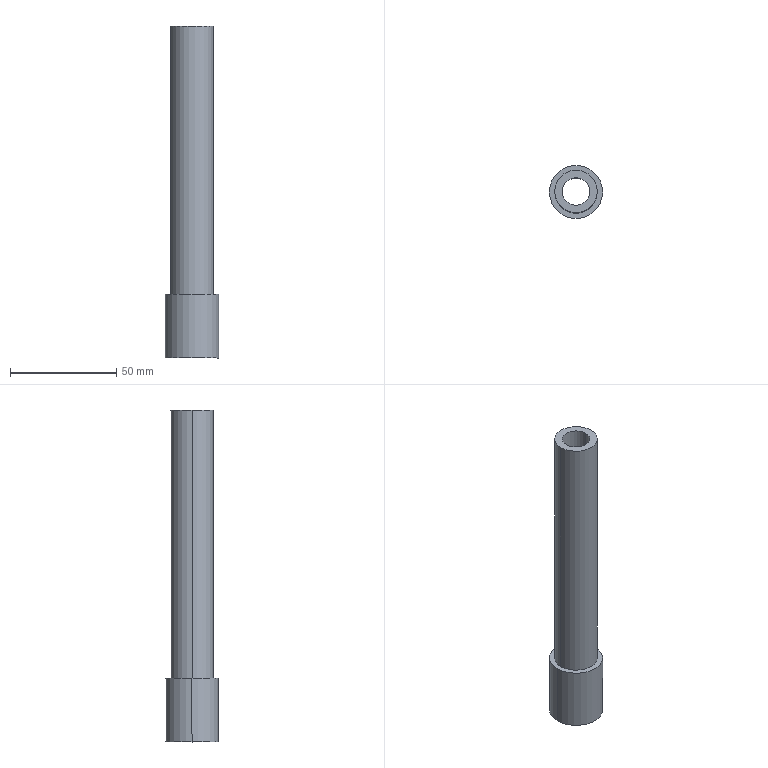Part | SolidWorks | features BaseBody 1 | 1 solid | 9 faces | box 25 x 25 x 156 mm | volume 33604 mm3 | cylinder 6 | plane 3 | commonest cylinder face diameters 13 x2 20 x2 25 x2
STEP:
#1=CARTESIAN_POINT('',(6.5,0.,78.));
#2=VERTEX_POINT('',#1);
#3=CARTESIAN_POINT('',(6.5,0.,-78.));
#4=VERTEX_POINT('',#3);
#5=CARTESIAN_POINT('',(6.5,0.,78.));
#6=DIRECTION('',(0.,0.,-1.));
#7=VECTOR('',#6,1000.);
#8=LINE('',#5,#7);
#9=EDGE_CURVE('',#2,#4,#8,.T.);
#10=ORIENTED_EDGE('',*,*,#9,.F.);
#11=CARTESIAN_POINT('',(-6.5,0.,78.));
#12=VERTEX_POINT('',#11);
#13=CARTESIAN_POINT('',(0.,0.,78.));
#14=DIRECTION('',(0.,0.,-1.));
#15=DIRECTION('',(-1.,0.,0.));
#16=AXIS2_PLACEMENT_3D('',#13,#14,#15);
#17=CIRCLE('',#16,6.5);
#18=EDGE_CURVE('',#12,#2,#17,.T.);
#19=ORIENTED_EDGE('',*,*,#18,.F.);
#20=CARTESIAN_POINT('',(-6.5,0.,-78.));
#21=VERTEX_POINT('',#20);
#22=CARTESIAN_POINT('',(-6.5,0.,78.));
#23=DIRECTION('',(0.,0.,-1.));
#24=VECTOR('',#23,1000.);
#25=LINE('',#22,#24);
#26=EDGE_CURVE('',#12,#21,#25,.T.);
#27=ORIENTED_EDGE('',*,*,#26,.T.);
#28=CARTESIAN_POINT('',(0.,0.,-78.));
#29=DIRECTION('',(0.,0.,-1.));
#30=DIRECTION('',(-1.,0.,0.));
#31=AXIS2_PLACEMENT_3D('',#28,#29,#30);
#32=CIRCLE('',#31,6.5);
#33=EDGE_CURVE('',#21,#4,#32,.T.);
#34=ORIENTED_EDGE('',*,*,#33,.T.);
#35=EDGE_LOOP('',(#10,#19,#27,#34));
#36=FACE_OUTER_BOUND('',#35,.T.);
#37=CARTESIAN_POINT('',(0.,0.,78.));
#38=DIRECTION('',(0.,0.,-1.));
#39=DIRECTION('',(-1.,0.,0.));
#40=AXIS2_PLACEMENT_3D('',#37,#38,#39);
#41=CYLINDRICAL_SURFACE('',#40,6.5);
#42=ADVANCED_FACE('',(#36),#41,.F.);
#43=ORIENTED_EDGE('',*,*,#33,.F.);
#44=CARTESIAN_POINT('',(0.,0.,-78.));
#45=DIRECTION('',(0.,0.,-1.));
#46=DIRECTION('',(-1.,0.,0.));
#47=AXIS2_PLACEMENT_3D('',#44,#45,#46);
#48=CIRCLE('',#47,6.5);
#49=EDGE_CURVE('',#4,#21,#48,.T.);
#50=ORIENTED_EDGE('',*,*,#49,.F.);
#51=EDGE_LOOP('',(#43,#50));
#52=FACE_BOUND('',#51,.T.);
#53=CARTESIAN_POINT('',(-12.5,0.,-78.));
#54=VERTEX_POINT('',#53);
#55=CARTESIAN_POINT('',(12.5,0.,-78.));
#56=VERTEX_POINT('',#55);
#57=CARTESIAN_POINT('',(0.,0.,-78.));
#58=DIRECTION('',(0.,0.,-1.));
#59=DIRECTION('',(-1.,0.,0.));
#60=AXIS2_PLACEMENT_3D('',#57,#58,#59);
#61=CIRCLE('',#60,12.5);
#62=EDGE_CURVE('',#54,#56,#61,.T.);
#63=ORIENTED_EDGE('',*,*,#62,.T.);
#64=CARTESIAN_POINT('',(0.,0.,-78.));
#65=DIRECTION('',(0.,0.,-1.));
#66=DIRECTION('',(-1.,0.,0.));
#67=AXIS2_PLACEMENT_3D('',#64,#65,#66);
#68=CIRCLE('',#67,12.5);
#69=EDGE_CURVE('',#56,#54,#68,.T.);
#70=ORIENTED_EDGE('',*,*,#69,.T.);
#71=EDGE_LOOP('',(#63,#70));
#72=FACE_OUTER_BOUND('',#71,.T.);
#73=CARTESIAN_POINT('',(0.,0.,-78.));
#74=DIRECTION('',(0.,0.,1.));
#75=DIRECTION('',(1.,0.,0.));
#76=AXIS2_PLACEMENT_3D('',#73,#74,#75);
#77=PLANE('',#76);
#78=ADVANCED_FACE('',(#52,#72),#77,.F.);
#79=CARTESIAN_POINT('',(-10.,0.,-48.));
#80=VERTEX_POINT('',#79);
#81=CARTESIAN_POINT('',(10.,0.,-48.));
#82=VERTEX_POINT('',#81);
#83=CARTESIAN_POINT('',(0.,0.,-48.));
#84=DIRECTION('',(0.,0.,-1.));
#85=DIRECTION('',(-1.,0.,0.));
#86=AXIS2_PLACEMENT_3D('',#83,#84,#85);
#87=CIRCLE('',#86,10.);
#88=EDGE_CURVE('',#80,#82,#87,.T.);
#89=ORIENTED_EDGE('',*,*,#88,.T.);
#90=CARTESIAN_POINT('',(0.,0.,-48.));
#91=DIRECTION('',(0.,0.,-1.));
#92=DIRECTION('',(-1.,0.,0.));
#93=AXIS2_PLACEMENT_3D('',#90,#91,#92);
#94=CIRCLE('',#93,10.);
#95=EDGE_CURVE('',#82,#80,#94,.T.);
#96=ORIENTED_EDGE('',*,*,#95,.T.);
#97=EDGE_LOOP('',(#89,#96));
#98=FACE_BOUND('',#97,.T.);
#99=CARTESIAN_POINT('',(-12.5,0.,-48.));
#100=VERTEX_POINT('',#99);
#101=CARTESIAN_POINT('',(12.5,0.,-48.));
#102=VERTEX_POINT('',#101);
#103=CARTESIAN_POINT('',(0.,0.,-48.));
#104=DIRECTION('',(0.,0.,-1.));
#105=DIRECTION('',(-1.,0.,0.));
#106=AXIS2_PLACEMENT_3D('',#103,#104,#105);
#107=CIRCLE('',#106,12.5);
#108=EDGE_CURVE('',#100,#102,#107,.T.);
#109=ORIENTED_EDGE('',*,*,#108,.F.);
#110=CARTESIAN_POINT('',(0.,0.,-48.));
#111=DIRECTION('',(0.,0.,-1.));
#112=DIRECTION('',(-1.,0.,0.));
#113=AXIS2_PLACEMENT_3D('',#110,#111,#112);
#114=CIRCLE('',#113,12.5);
#115=EDGE_CURVE('',#102,#100,#114,.T.);
#116=ORIENTED_EDGE('',*,*,#115,.F.);
#117=EDGE_LOOP('',(#109,#116));
#118=FACE_OUTER_BOUND('',#117,.T.);
#119=CARTESIAN_POINT('',(0.,0.,-48.));
#120=DIRECTION('',(0.,0.,-1.));
#121=DIRECTION('',(0.,-1.,0.));
#122=AXIS2_PLACEMENT_3D('',#119,#120,#121);
#123=PLANE('',#122);
#124=ADVANCED_FACE('',(#98,#118),#123,.F.);
#125=CARTESIAN_POINT('',(12.5,0.,-48.));
#126=DIRECTION('',(0.,0.,-1.));
#127=VECTOR('',#126,1000.);
#128=LINE('',#125,#127);
#129=EDGE_CURVE('',#102,#56,#128,.T.);
#130=ORIENTED_EDGE('',*,*,#129,.F.);
#131=ORIENTED_EDGE('',*,*,#115,.T.);
#132=CARTESIAN_POINT('',(-12.5,0.,-48.));
#133=DIRECTION('',(0.,0.,-1.));
#134=VECTOR('',#133,1000.);
#135=LINE('',#132,#134);
#136=EDGE_CURVE('',#100,#54,#135,.T.);
#137=ORIENTED_EDGE('',*,*,#136,.T.);
#138=ORIENTED_EDGE('',*,*,#69,.F.);
#139=EDGE_LOOP('',(#130,#131,#137,#138));
#140=FACE_OUTER_BOUND('',#139,.T.);
#141=CARTESIAN_POINT('',(0.,0.,-48.));
#142=DIRECTION('',(0.,0.,-1.));
#143=DIRECTION('',(-1.,0.,0.));
#144=AXIS2_PLACEMENT_3D('',#141,#142,#143);
#145=CYLINDRICAL_SURFACE('',#144,12.5);
#146=ADVANCED_FACE('',(#140),#145,.T.);
#147=ORIENTED_EDGE('',*,*,#18,.T.);
#148=CARTESIAN_POINT('',(0.,0.,78.));
#149=DIRECTION('',(0.,0.,-1.));
#150=DIRECTION('',(-1.,0.,0.));
#151=AXIS2_PLACEMENT_3D('',#148,#149,#150);
#152=CIRCLE('',#151,6.5);
#153=EDGE_CURVE('',#2,#12,#152,.T.);
#154=ORIENTED_EDGE('',*,*,#153,.T.);
#155=EDGE_LOOP('',(#147,#154));
#156=FACE_BOUND('',#155,.T.);
#157=CARTESIAN_POINT('',(-10.,0.,78.));
#158=VERTEX_POINT('',#157);
#159=CARTESIAN_POINT('',(10.,0.,78.));
#160=VERTEX_POINT('',#159);
#161=CARTESIAN_POINT('',(0.,0.,78.));
#162=DIRECTION('',(0.,0.,1.));
#163=DIRECTION('',(1.,0.,0.));
#164=AXIS2_PLACEMENT_3D('',#161,#162,#163);
#165=CIRCLE('',#164,10.);
#166=EDGE_CURVE('',#158,#160,#165,.T.);
#167=ORIENTED_EDGE('',*,*,#166,.T.);
#168=CARTESIAN_POINT('',(0.,0.,78.));
#169=DIRECTION('',(0.,0.,1.));
#170=DIRECTION('',(1.,0.,0.));
#171=AXIS2_PLACEMENT_3D('',#168,#169,#170);
#172=CIRCLE('',#171,10.);
#173=EDGE_CURVE('',#160,#158,#172,.T.);
#174=ORIENTED_EDGE('',*,*,#173,.T.);
#175=EDGE_LOOP('',(#167,#174));
#176=FACE_OUTER_BOUND('',#175,.T.);
#177=CARTESIAN_POINT('',(0.,0.,78.));
#178=DIRECTION('',(0.,0.,1.));
#179=DIRECTION('',(1.,0.,0.));
#180=AXIS2_PLACEMENT_3D('',#177,#178,#179);
#181=PLANE('',#180);
#182=ADVANCED_FACE('',(#156,#176),#181,.T.);
#183=CARTESIAN_POINT('',(10.,0.,78.));
#184=DIRECTION('',(0.,0.,-1.));
#185=VECTOR('',#184,1000.);
#186=LINE('',#183,#185);
#187=EDGE_CURVE('',#160,#82,#186,.T.);
#188=ORIENTED_EDGE('',*,*,#187,.F.);
#189=ORIENTED_EDGE('',*,*,#166,.F.);
#190=CARTESIAN_POINT('',(-10.,0.,78.));
#191=DIRECTION('',(0.,0.,-1.));
#192=VECTOR('',#191,1000.);
#193=LINE('',#190,#192);
#194=EDGE_CURVE('',#158,#80,#193,.T.);
#195=ORIENTED_EDGE('',*,*,#194,.T.);
#196=ORIENTED_EDGE('',*,*,#95,.F.);
#197=EDGE_LOOP('',(#188,#189,#195,#196));
#198=FACE_OUTER_BOUND('',#197,.T.);
#199=CARTESIAN_POINT('',(0.,0.,78.));
#200=DIRECTION('',(0.,0.,-1.));
#201=DIRECTION('',(-1.,0.,0.));
#202=AXIS2_PLACEMENT_3D('',#199,#200,#201);
#203=CYLINDRICAL_SURFACE('',#202,10.);
#204=ADVANCED_FACE('',(#198),#203,.T.);
#205=ORIENTED_EDGE('',*,*,#173,.F.);
#206=ORIENTED_EDGE('',*,*,#187,.T.);
#207=ORIENTED_EDGE('',*,*,#88,.F.);
#208=ORIENTED_EDGE('',*,*,#194,.F.);
#209=EDGE_LOOP('',(#205,#206,#207,#208));
#210=FACE_OUTER_BOUND('',#209,.T.);
#211=CARTESIAN_POINT('',(0.,0.,78.));
#212=DIRECTION('',(0.,0.,-1.));
#213=DIRECTION('',(-1.,0.,0.));
#214=AXIS2_PLACEMENT_3D('',#211,#212,#213);
#215=CYLINDRICAL_SURFACE('',#214,10.);
#216=ADVANCED_FACE('',(#210),#215,.T.);
#217=ORIENTED_EDGE('',*,*,#108,.T.);
#218=ORIENTED_EDGE('',*,*,#129,.T.);
#219=ORIENTED_EDGE('',*,*,#62,.F.);
#220=ORIENTED_EDGE('',*,*,#136,.F.);
#221=EDGE_LOOP('',(#217,#218,#219,#220));
#222=FACE_OUTER_BOUND('',#221,.T.);
#223=CARTESIAN_POINT('',(0.,0.,-48.));
#224=DIRECTION('',(0.,0.,-1.));
#225=DIRECTION('',(-1.,0.,0.));
#226=AXIS2_PLACEMENT_3D('',#223,#224,#225);
#227=CYLINDRICAL_SURFACE('',#226,12.5);
#228=ADVANCED_FACE('',(#222),#227,.T.);
#229=ORIENTED_EDGE('',*,*,#153,.F.);
#230=ORIENTED_EDGE('',*,*,#9,.T.);
#231=ORIENTED_EDGE('',*,*,#49,.T.);
#232=ORIENTED_EDGE('',*,*,#26,.F.);
#233=EDGE_LOOP('',(#229,#230,#231,#232));
#234=FACE_OUTER_BOUND('',#233,.T.);
#235=CARTESIAN_POINT('',(0.,0.,78.));
#236=DIRECTION('',(0.,0.,-1.));
#237=DIRECTION('',(-1.,0.,0.));
#238=AXIS2_PLACEMENT_3D('',#235,#236,#237);
#239=CYLINDRICAL_SURFACE('',#238,6.5);
#240=ADVANCED_FACE('',(#234),#239,.F.);
#241=CLOSED_SHELL('',(#42,#78,#124,#146,#182,#204,#216,#228,#240));
#242=MANIFOLD_SOLID_BREP('',#241);
#243=CARTESIAN_POINT('',(0.,0.,0.));
#244=DIRECTION('',(0.,0.,1.));
#245=DIRECTION('',(1.,0.,0.));
#246=AXIS2_PLACEMENT_3D('',#243,#244,#245);
#247=(LENGTH_UNIT()NAMED_UNIT(*)SI_UNIT(.MILLI.,.METRE.));
#248=UNCERTAINTY_MEASURE_WITH_UNIT(LENGTH_MEASURE(0.00001),#247,'','');
#249=(NAMED_UNIT(*)PLANE_ANGLE_UNIT()SI_UNIT($,.RADIAN.));
#250=(NAMED_UNIT(*)SI_UNIT($,.STERADIAN.)SOLID_ANGLE_UNIT());
#251=(GEOMETRIC_REPRESENTATION_CONTEXT(3)GLOBAL_UNCERTAINTY_ASSIGNED_CONTEXT((#248))GLOBAL_UNIT_ASSIGNED_CONTEXT((#247,#249,#250))REPRESENTATION_CONTEXT('',''));
#252=ADVANCED_BREP_SHAPE_REPRESENTATION('',(#242,#246),#251);